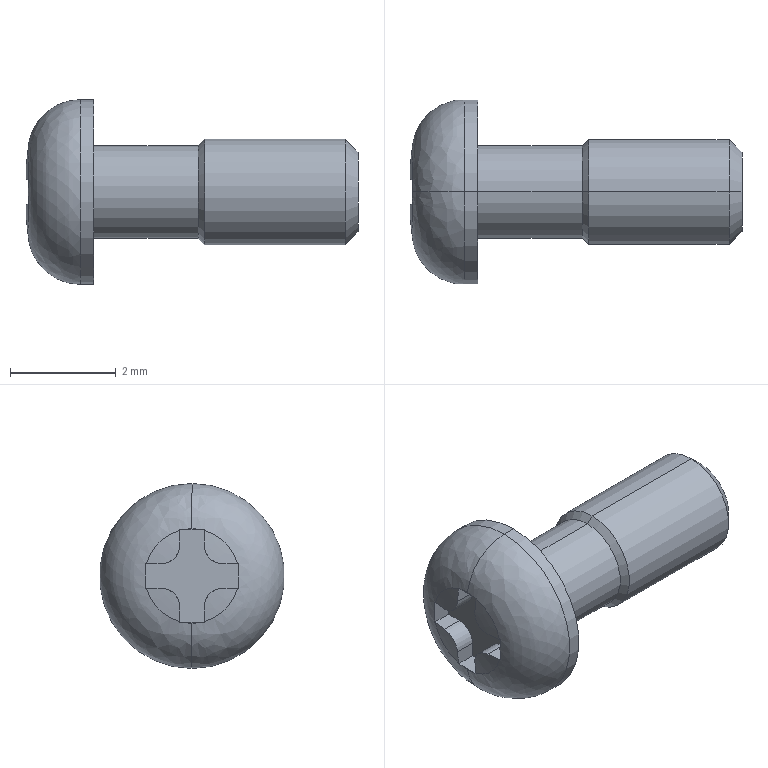Part | STEP file | 0232_Z_SCBJ2-5_1 | 1 solid | 37 faces | box 6.282 x 3.5 x 3.5 mm | volume 23.426 mm3 | plane 15 | cylinder 10 | spline 8 | cone 4 | commonest cylinder face diameters 0.7 x4 1.754 x2 2 x2 3.5 x2